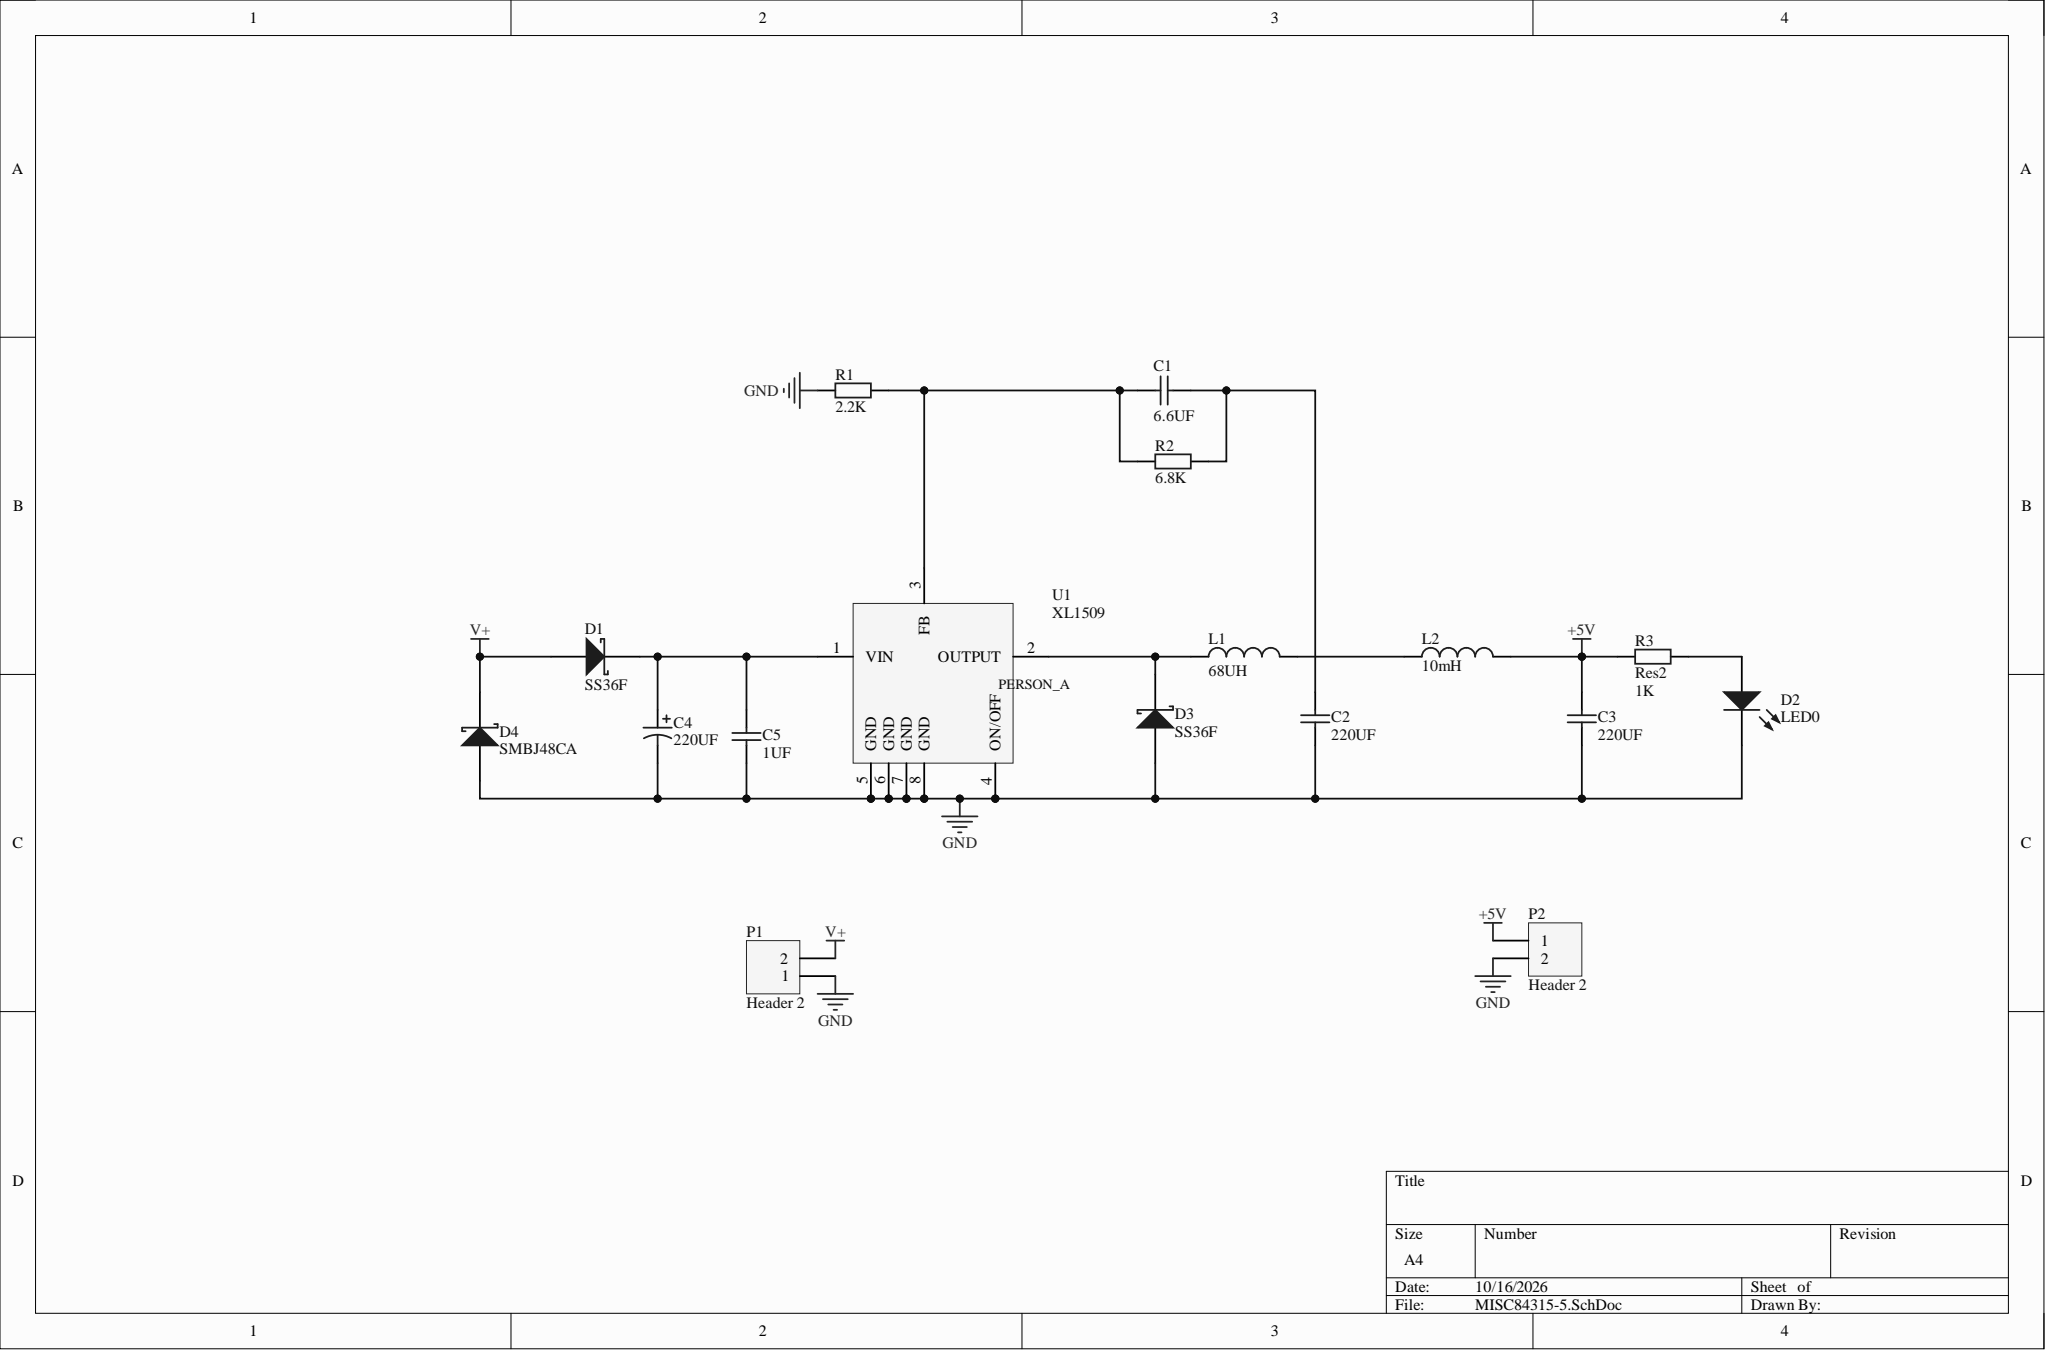Circuit board | Altium Designer | 17 parts | 9 nets
Bill of materials:
Comment,Description,Designator,Footprint,LibRef,Quantity
"6.6UF","Capacitor","C1","C0805","Cap","1"
"220UF","Capacitor","C2, C3","C0805","Cap","2"
"220UF","Polarized Capacitor (Radial)","C4","RAD-0.4","Cap Pol1","1"
"1UF","Capacitor","C5","C0805","Cap","1"
"SS36F","Schottky Diode","D1, D3","C1206","D Schottky","2"
"LED0","Typical INFRARED GaAs LED","D2","LED-0","LED0","1"
"SMBJ48CA","Schottky Diode","D4","C1206","D Schottky","1"
"68UH","Inductor","L1","INDC1608L","Inductor","1"
"Inductor","Inductor","L2","INDC1608L","Inductor","1"
"Header 2","Header, 2-Pin","P1, P2","HDR1X2","Header 2","2"
"2.2K","Resistor","R1","C0805","Res2","1"
"6.8K","Resistor","R2","C0805","Res2","1"
"Res2","Resistor","R3","C0805","Res2","1"
"XL1509","","U1","ESOP8","XL1509","1"
Netlist (Protel format):
[
C1
C0805
6.6UF



]
[
C2
C0805
220UF



]
[
C3
C0805
220UF



]
[
C4
RAD-0.4
220UF



]
[
C5
C0805
1UF



]
[
D1
C1206
SS36F



]
[
D2
LED-0
LED0



]
[
D3
C1206
SS36F



]
[
D4
C1206
SMBJ48CA



]
[
L1
INDC1608L
68UH



]
[
L2
INDC1608L
Inductor



]
[
P1
HDR1X2
Header 2



]
[
P2
HDR1X2
Header 2



]
[
R1
C0805
2.2K



]
[
R2
C0805
6.8K



]
[
R3
C0805
Res2



]
[
U1
ESOP8
XL1509



]
(
V+
D1-1
D4-2
P1-2
)
(
NetL1_2
L1-2
L2-1
)
(
NetD3_2
D3-2
L1-1
U1-2
)
(
NetD2_1
D2-1
R3-2
)
(
NetC4_1
C4-1
C5-2
D1-2
U1-1
)
(
NetC1_2
C1-2
C2-2
R2-2
)
(
NetC1_1
C1-1
R1-2
R2-1
U1-3
)
(
GND
C2-1
C3-1
C4-2
C5-1
D2-2
D3-1
D4-1
P1-1
P2-2
R1-1
U1-4
U1-5
U1-6
U1-7
U1-8
)
(
+5V
C3-2
L2-2
P2-1
R3-1
)